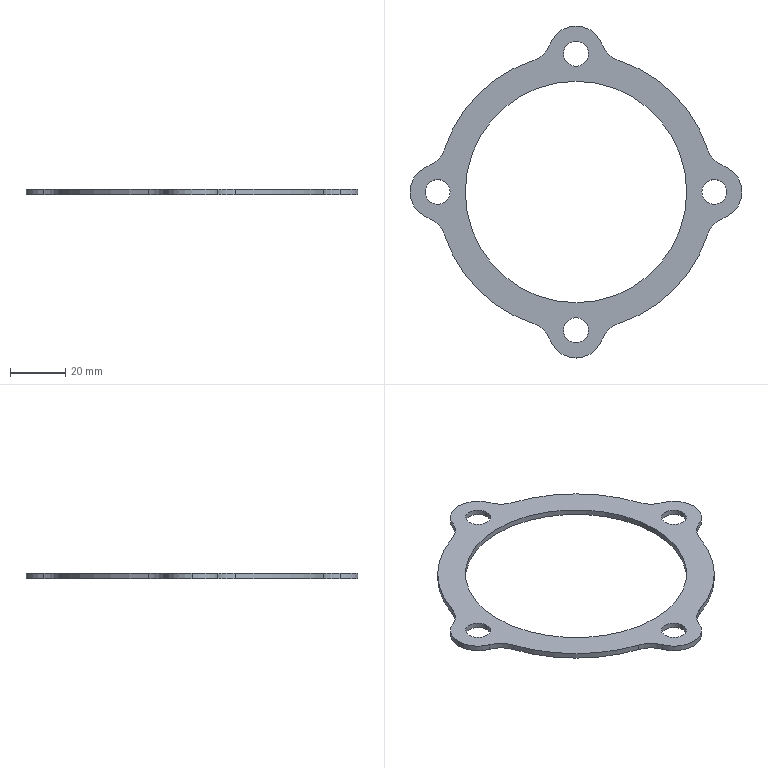Part | STEP file | USZCZELKA1V11 | 1 solid | 29 faces | box 120 x 120 x 2 mm | volume 6543 mm3 | cylinder 27 | plane 2 | commonest cylinder face diameters 20 x13 9 x8 100 x4 80 x2